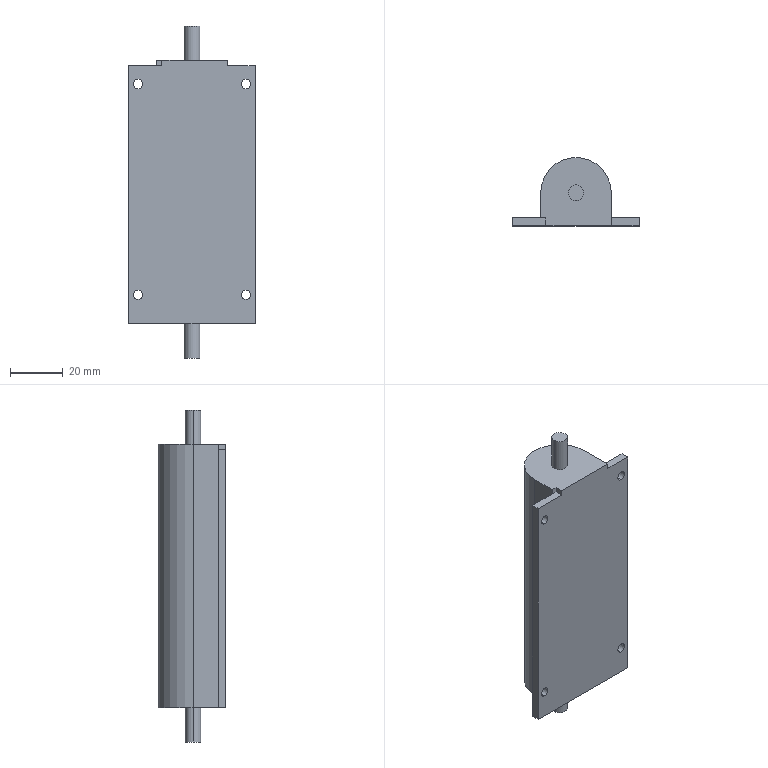Part | SolidWorks | features ICE 7, Extrusion 1 | 1 solid | 28 faces | box 48 x 25.9 x 126 mm | volume 68546 mm3 | plane 15 | cylinder 13 | commonest cylinder face diameters 3.5 x8 6 x4 26.8 x1
STEP:
#1=CARTESIAN_POINT('',(-20.5,3.,-38.25));
#2=VERTEX_POINT('',#1);
#3=CARTESIAN_POINT('',(-20.5,3.,-41.75));
#4=VERTEX_POINT('',#3);
#5=CARTESIAN_POINT('',(-20.5,3.,-40.));
#6=DIRECTION('',(0.,-1.,0.));
#7=DIRECTION('',(1.,0.,0.));
#8=AXIS2_PLACEMENT_3D('',#5,#6,#7);
#9=CIRCLE('',#8,1.75);
#10=EDGE_CURVE('',#2,#4,#9,.T.);
#11=ORIENTED_EDGE('',*,*,#10,.F.);
#12=CARTESIAN_POINT('',(-20.5,0.,-38.25));
#13=VERTEX_POINT('',#12);
#14=CARTESIAN_POINT('',(-20.5,10.,-38.25));
#15=DIRECTION('',(0.,-1.,0.));
#16=VECTOR('',#15,1000.);
#17=LINE('',#14,#16);
#18=EDGE_CURVE('',#2,#13,#17,.T.);
#19=ORIENTED_EDGE('',*,*,#18,.T.);
#20=CARTESIAN_POINT('',(-20.5,0.,-41.75));
#21=VERTEX_POINT('',#20);
#22=CARTESIAN_POINT('',(-20.5,0.,-40.));
#23=DIRECTION('',(0.,-1.,0.));
#24=DIRECTION('',(0.,0.,-1.));
#25=AXIS2_PLACEMENT_3D('',#22,#23,#24);
#26=CIRCLE('',#25,1.75);
#27=EDGE_CURVE('',#13,#21,#26,.T.);
#28=ORIENTED_EDGE('',*,*,#27,.T.);
#29=CARTESIAN_POINT('',(-20.5,10.,-41.75));
#30=DIRECTION('',(0.,-1.,0.));
#31=VECTOR('',#30,1000.);
#32=LINE('',#29,#31);
#33=EDGE_CURVE('',#4,#21,#32,.T.);
#34=ORIENTED_EDGE('',*,*,#33,.F.);
#35=EDGE_LOOP('',(#11,#19,#28,#34));
#36=FACE_OUTER_BOUND('',#35,.T.);
#37=CARTESIAN_POINT('',(-20.5,10.,-40.));
#38=DIRECTION('',(0.,-1.,0.));
#39=DIRECTION('',(0.,0.,-1.));
#40=AXIS2_PLACEMENT_3D('',#37,#38,#39);
#41=CYLINDRICAL_SURFACE('',#40,1.75);
#42=ADVANCED_FACE('',(#36),#41,.F.);
#43=CARTESIAN_POINT('',(20.5,3.,-38.25));
#44=VERTEX_POINT('',#43);
#45=CARTESIAN_POINT('',(20.5,3.,-41.75));
#46=VERTEX_POINT('',#45);
#47=CARTESIAN_POINT('',(20.5,3.,-40.));
#48=DIRECTION('',(0.,-1.,0.));
#49=DIRECTION('',(0.,0.,-1.));
#50=AXIS2_PLACEMENT_3D('',#47,#48,#49);
#51=CIRCLE('',#50,1.75);
#52=EDGE_CURVE('',#44,#46,#51,.T.);
#53=ORIENTED_EDGE('',*,*,#52,.F.);
#54=CARTESIAN_POINT('',(20.5,0.,-38.25));
#55=VERTEX_POINT('',#54);
#56=CARTESIAN_POINT('',(20.5,10.,-38.25));
#57=DIRECTION('',(0.,-1.,0.));
#58=VECTOR('',#57,1000.);
#59=LINE('',#56,#58);
#60=EDGE_CURVE('',#44,#55,#59,.T.);
#61=ORIENTED_EDGE('',*,*,#60,.T.);
#62=CARTESIAN_POINT('',(20.5,0.,-41.75));
#63=VERTEX_POINT('',#62);
#64=CARTESIAN_POINT('',(20.5,0.,-40.));
#65=DIRECTION('',(0.,-1.,0.));
#66=DIRECTION('',(0.,0.,-1.));
#67=AXIS2_PLACEMENT_3D('',#64,#65,#66);
#68=CIRCLE('',#67,1.75);
#69=EDGE_CURVE('',#55,#63,#68,.T.);
#70=ORIENTED_EDGE('',*,*,#69,.T.);
#71=CARTESIAN_POINT('',(20.5,10.,-41.75));
#72=DIRECTION('',(0.,-1.,0.));
#73=VECTOR('',#72,1000.);
#74=LINE('',#71,#73);
#75=EDGE_CURVE('',#46,#63,#74,.T.);
#76=ORIENTED_EDGE('',*,*,#75,.F.);
#77=EDGE_LOOP('',(#53,#61,#70,#76));
#78=FACE_OUTER_BOUND('',#77,.T.);
#79=CARTESIAN_POINT('',(20.5,10.,-40.));
#80=DIRECTION('',(0.,-1.,0.));
#81=DIRECTION('',(0.,0.,-1.));
#82=AXIS2_PLACEMENT_3D('',#79,#80,#81);
#83=CYLINDRICAL_SURFACE('',#82,1.75);
#84=ADVANCED_FACE('',(#78),#83,.F.);
#85=CARTESIAN_POINT('',(20.5,3.,41.75));
#86=VERTEX_POINT('',#85);
#87=CARTESIAN_POINT('',(20.5,3.,38.25));
#88=VERTEX_POINT('',#87);
#89=CARTESIAN_POINT('',(20.5,3.,40.));
#90=DIRECTION('',(0.,-1.,0.));
#91=DIRECTION('',(0.,0.,-1.));
#92=AXIS2_PLACEMENT_3D('',#89,#90,#91);
#93=CIRCLE('',#92,1.75);
#94=EDGE_CURVE('',#86,#88,#93,.T.);
#95=ORIENTED_EDGE('',*,*,#94,.F.);
#96=CARTESIAN_POINT('',(20.5,0.,41.75));
#97=VERTEX_POINT('',#96);
#98=CARTESIAN_POINT('',(20.5,10.,41.75));
#99=DIRECTION('',(0.,-1.,0.));
#100=VECTOR('',#99,1000.);
#101=LINE('',#98,#100);
#102=EDGE_CURVE('',#86,#97,#101,.T.);
#103=ORIENTED_EDGE('',*,*,#102,.T.);
#104=CARTESIAN_POINT('',(20.5,0.,38.25));
#105=VERTEX_POINT('',#104);
#106=CARTESIAN_POINT('',(20.5,0.,40.));
#107=DIRECTION('',(0.,-1.,0.));
#108=DIRECTION('',(0.,0.,-1.));
#109=AXIS2_PLACEMENT_3D('',#106,#107,#108);
#110=CIRCLE('',#109,1.75);
#111=EDGE_CURVE('',#97,#105,#110,.T.);
#112=ORIENTED_EDGE('',*,*,#111,.T.);
#113=CARTESIAN_POINT('',(20.5,10.,38.25));
#114=DIRECTION('',(0.,-1.,0.));
#115=VECTOR('',#114,1000.);
#116=LINE('',#113,#115);
#117=EDGE_CURVE('',#88,#105,#116,.T.);
#118=ORIENTED_EDGE('',*,*,#117,.F.);
#119=EDGE_LOOP('',(#95,#103,#112,#118));
#120=FACE_OUTER_BOUND('',#119,.T.);
#121=CARTESIAN_POINT('',(20.5,10.,40.));
#122=DIRECTION('',(0.,-1.,0.));
#123=DIRECTION('',(0.,0.,-1.));
#124=AXIS2_PLACEMENT_3D('',#121,#122,#123);
#125=CYLINDRICAL_SURFACE('',#124,1.75);
#126=ADVANCED_FACE('',(#120),#125,.F.);
#127=CARTESIAN_POINT('',(-20.5,3.,41.75));
#128=VERTEX_POINT('',#127);
#129=CARTESIAN_POINT('',(-20.5,3.,38.25));
#130=VERTEX_POINT('',#129);
#131=CARTESIAN_POINT('',(-20.5,3.,40.));
#132=DIRECTION('',(0.,-1.,0.));
#133=DIRECTION('',(1.,0.,0.));
#134=AXIS2_PLACEMENT_3D('',#131,#132,#133);
#135=CIRCLE('',#134,1.75);
#136=EDGE_CURVE('',#128,#130,#135,.T.);
#137=ORIENTED_EDGE('',*,*,#136,.F.);
#138=CARTESIAN_POINT('',(-20.5,0.,41.75));
#139=VERTEX_POINT('',#138);
#140=CARTESIAN_POINT('',(-20.5,10.,41.75));
#141=DIRECTION('',(0.,-1.,0.));
#142=VECTOR('',#141,1000.);
#143=LINE('',#140,#142);
#144=EDGE_CURVE('',#128,#139,#143,.T.);
#145=ORIENTED_EDGE('',*,*,#144,.T.);
#146=CARTESIAN_POINT('',(-20.5,0.,38.25));
#147=VERTEX_POINT('',#146);
#148=CARTESIAN_POINT('',(-20.5,0.,40.));
#149=DIRECTION('',(0.,-1.,0.));
#150=DIRECTION('',(0.,0.,-1.));
#151=AXIS2_PLACEMENT_3D('',#148,#149,#150);
#152=CIRCLE('',#151,1.75);
#153=EDGE_CURVE('',#139,#147,#152,.T.);
#154=ORIENTED_EDGE('',*,*,#153,.T.);
#155=CARTESIAN_POINT('',(-20.5,10.,38.25));
#156=DIRECTION('',(0.,-1.,0.));
#157=VECTOR('',#156,1000.);
#158=LINE('',#155,#157);
#159=EDGE_CURVE('',#130,#147,#158,.T.);
#160=ORIENTED_EDGE('',*,*,#159,.F.);
#161=EDGE_LOOP('',(#137,#145,#154,#160));
#162=FACE_OUTER_BOUND('',#161,.T.);
#163=CARTESIAN_POINT('',(-20.5,10.,40.));
#164=DIRECTION('',(0.,-1.,0.));
#165=DIRECTION('',(0.,0.,-1.));
#166=AXIS2_PLACEMENT_3D('',#163,#164,#165);
#167=CYLINDRICAL_SURFACE('',#166,1.75);
#168=ADVANCED_FACE('',(#162),#167,.F.);
#169=CARTESIAN_POINT('',(-3.,12.5,-64.));
#170=VERTEX_POINT('',#169);
#171=CARTESIAN_POINT('',(3.,12.5,-64.));
#172=VERTEX_POINT('',#171);
#173=CARTESIAN_POINT('',(0.,12.5,-64.));
#174=DIRECTION('',(0.,0.,-1.));
#175=DIRECTION('',(-1.,0.,0.));
#176=AXIS2_PLACEMENT_3D('',#173,#174,#175);
#177=CIRCLE('',#176,3.);
#178=EDGE_CURVE('',#170,#172,#177,.T.);
#179=ORIENTED_EDGE('',*,*,#178,.F.);
#180=CARTESIAN_POINT('',(-3.,12.5,-51.));
#181=VERTEX_POINT('',#180);
#182=CARTESIAN_POINT('',(-3.,12.5,-64.));
#183=DIRECTION('',(0.,0.,1.));
#184=VECTOR('',#183,1000.);
#185=LINE('',#182,#184);
#186=EDGE_CURVE('',#170,#181,#185,.T.);
#187=ORIENTED_EDGE('',*,*,#186,.T.);
#188=CARTESIAN_POINT('',(3.,12.5,-51.));
#189=VERTEX_POINT('',#188);
#190=CARTESIAN_POINT('',(0.,12.5,-51.));
#191=DIRECTION('',(0.,0.,-1.));
#192=DIRECTION('',(1.,0.,0.));
#193=AXIS2_PLACEMENT_3D('',#190,#191,#192);
#194=CIRCLE('',#193,3.);
#195=EDGE_CURVE('',#181,#189,#194,.T.);
#196=ORIENTED_EDGE('',*,*,#195,.T.);
#197=CARTESIAN_POINT('',(3.,12.5,-64.));
#198=DIRECTION('',(0.,0.,1.));
#199=VECTOR('',#198,1000.);
#200=LINE('',#197,#199);
#201=EDGE_CURVE('',#172,#189,#200,.T.);
#202=ORIENTED_EDGE('',*,*,#201,.F.);
#203=EDGE_LOOP('',(#179,#187,#196,#202));
#204=FACE_OUTER_BOUND('',#203,.T.);
#205=CARTESIAN_POINT('',(0.,12.5,-64.));
#206=DIRECTION('',(0.,0.,1.));
#207=DIRECTION('',(1.,0.,0.));
#208=AXIS2_PLACEMENT_3D('',#205,#206,#207);
#209=CYLINDRICAL_SURFACE('',#208,3.);
#210=ADVANCED_FACE('',(#204),#209,.T.);
#211=CARTESIAN_POINT('',(3.,12.5,62.));
#212=VERTEX_POINT('',#211);
#213=CARTESIAN_POINT('',(-3.,12.5,62.));
#214=VERTEX_POINT('',#213);
#215=CARTESIAN_POINT('',(0.,12.5,62.));
#216=DIRECTION('',(0.,0.,1.));
#217=DIRECTION('',(1.,0.,0.));
#218=AXIS2_PLACEMENT_3D('',#215,#216,#217);
#219=CIRCLE('',#218,3.);
#220=EDGE_CURVE('',#212,#214,#219,.T.);
#221=ORIENTED_EDGE('',*,*,#220,.F.);
#222=CARTESIAN_POINT('',(3.,12.5,49.));
#223=VERTEX_POINT('',#222);
#224=CARTESIAN_POINT('',(3.,12.5,62.));
#225=DIRECTION('',(0.,0.,-1.));
#226=VECTOR('',#225,1000.);
#227=LINE('',#224,#226);
#228=EDGE_CURVE('',#212,#223,#227,.T.);
#229=ORIENTED_EDGE('',*,*,#228,.T.);
#230=CARTESIAN_POINT('',(-3.,12.5,49.));
#231=VERTEX_POINT('',#230);
#232=CARTESIAN_POINT('',(0.,12.5,49.));
#233=DIRECTION('',(0.,0.,1.));
#234=DIRECTION('',(1.,0.,0.));
#235=AXIS2_PLACEMENT_3D('',#232,#233,#234);
#236=CIRCLE('',#235,3.);
#237=EDGE_CURVE('',#223,#231,#236,.T.);
#238=ORIENTED_EDGE('',*,*,#237,.T.);
#239=CARTESIAN_POINT('',(-3.,12.5,62.));
#240=DIRECTION('',(0.,0.,-1.));
#241=VECTOR('',#240,1000.);
#242=LINE('',#239,#241);
#243=EDGE_CURVE('',#214,#231,#242,.T.);
#244=ORIENTED_EDGE('',*,*,#243,.F.);
#245=EDGE_LOOP('',(#221,#229,#238,#244));
#246=FACE_OUTER_BOUND('',#245,.T.);
#247=CARTESIAN_POINT('',(0.,12.5,62.));
#248=DIRECTION('',(0.,0.,-1.));
#249=DIRECTION('',(-1.,0.,0.));
#250=AXIS2_PLACEMENT_3D('',#247,#248,#249);
#251=CYLINDRICAL_SURFACE('',#250,3.);
#252=ADVANCED_FACE('',(#246),#251,.T.);
#253=CARTESIAN_POINT('',(-24.,3.,-51.));
#254=VERTEX_POINT('',#253);
#255=CARTESIAN_POINT('',(-24.,0.,-51.));
#256=VERTEX_POINT('',#255);
#257=CARTESIAN_POINT('',(-24.,0.,-51.));
#258=DIRECTION('',(0.,-1.,0.));
#259=VECTOR('',#258,1000.);
#260=LINE('',#257,#259);
#261=EDGE_CURVE('',#254,#256,#260,.T.);
#262=ORIENTED_EDGE('',*,*,#261,.F.);
#263=CARTESIAN_POINT('',(-13.4,3.,-51.));
#264=VERTEX_POINT('',#263);
#265=CARTESIAN_POINT('',(-13.4,3.,-51.));
#266=DIRECTION('',(-1.,0.,0.));
#267=VECTOR('',#266,1000.);
#268=LINE('',#265,#267);
#269=EDGE_CURVE('',#264,#254,#268,.T.);
#270=ORIENTED_EDGE('',*,*,#269,.F.);
#271=CARTESIAN_POINT('',(-13.4,12.5,-51.));
#272=VERTEX_POINT('',#271);
#273=CARTESIAN_POINT('',(-13.4,12.5,-51.));
#274=DIRECTION('',(0.,-1.,0.));
#275=VECTOR('',#274,1000.);
#276=LINE('',#273,#275);
#277=EDGE_CURVE('',#272,#264,#276,.T.);
#278=ORIENTED_EDGE('',*,*,#277,.F.);
#279=CARTESIAN_POINT('',(13.4,12.5,-51.));
#280=VERTEX_POINT('',#279);
#281=CARTESIAN_POINT('',(0.,12.5,-51.));
#282=DIRECTION('',(0.,0.,1.));
#283=DIRECTION('',(1.,0.,0.));
#284=AXIS2_PLACEMENT_3D('',#281,#282,#283);
#285=CIRCLE('',#284,13.4);
#286=EDGE_CURVE('',#280,#272,#285,.T.);
#287=ORIENTED_EDGE('',*,*,#286,.F.);
#288=CARTESIAN_POINT('',(13.4,3.,-51.));
#289=VERTEX_POINT('',#288);
#290=CARTESIAN_POINT('',(13.4,0.,-51.));
#291=DIRECTION('',(0.,1.,0.));
#292=VECTOR('',#291,1000.);
#293=LINE('',#290,#292);
#294=EDGE_CURVE('',#289,#280,#293,.T.);
#295=ORIENTED_EDGE('',*,*,#294,.F.);
#296=CARTESIAN_POINT('',(24.,3.,-51.));
#297=VERTEX_POINT('',#296);
#298=CARTESIAN_POINT('',(24.,3.,-51.));
#299=DIRECTION('',(-1.,0.,0.));
#300=VECTOR('',#299,1000.);
#301=LINE('',#298,#300);
#302=EDGE_CURVE('',#297,#289,#301,.T.);
#303=ORIENTED_EDGE('',*,*,#302,.F.);
#304=CARTESIAN_POINT('',(24.,0.,-51.));
#305=VERTEX_POINT('',#304);
#306=CARTESIAN_POINT('',(24.,3.,-51.));
#307=DIRECTION('',(0.,1.,0.));
#308=VECTOR('',#307,1000.);
#309=LINE('',#306,#308);
#310=EDGE_CURVE('',#305,#297,#309,.T.);
#311=ORIENTED_EDGE('',*,*,#310,.F.);
#312=CARTESIAN_POINT('',(-13.4,0.,-51.));
#313=DIRECTION('',(1.,0.,0.));
#314=VECTOR('',#313,1000.);
#315=LINE('',#312,#314);
#316=EDGE_CURVE('',#256,#305,#315,.T.);
#317=ORIENTED_EDGE('',*,*,#316,.F.);
#318=EDGE_LOOP('',(#262,#270,#278,#287,#295,#303,#311,#317));
#319=FACE_OUTER_BOUND('',#318,.T.);
#320=CARTESIAN_POINT('',(0.,12.5,-51.));
#321=DIRECTION('',(0.,0.,-1.));
#322=DIRECTION('',(1.,0.,0.));
#323=AXIS2_PLACEMENT_3D('',#320,#321,#322);
#324=CIRCLE('',#323,3.);
#325=EDGE_CURVE('',#189,#181,#324,.T.);
#326=ORIENTED_EDGE('',*,*,#325,.F.);
#327=ORIENTED_EDGE('',*,*,#195,.F.);
#328=EDGE_LOOP('',(#326,#327));
#329=FACE_BOUND('',#328,.T.);
#330=CARTESIAN_POINT('',(0.,12.5,-51.));
#331=DIRECTION('',(0.,0.,1.));
#332=DIRECTION('',(1.,0.,0.));
#333=AXIS2_PLACEMENT_3D('',#330,#331,#332);
#334=PLANE('',#333);
#335=ADVANCED_FACE('',(#319,#329),#334,.F.);
#336=CARTESIAN_POINT('',(-11.4,3.,49.));
#337=VERTEX_POINT('',#336);
#338=CARTESIAN_POINT('',(-13.4,3.,49.));
#339=VERTEX_POINT('',#338);
#340=CARTESIAN_POINT('',(-11.4,3.,49.));
#341=DIRECTION('',(-1.,0.,0.));
#342=VECTOR('',#341,1000.);
#343=LINE('',#340,#342);
#344=EDGE_CURVE('',#337,#339,#343,.T.);
#345=ORIENTED_EDGE('',*,*,#344,.F.);
#346=CARTESIAN_POINT('',(-11.4,0.,49.));
#347=VERTEX_POINT('',#346);
#348=CARTESIAN_POINT('',(-11.4,12.5,49.));
#349=DIRECTION('',(0.,1.,0.));
#350=VECTOR('',#349,1000.);
#351=LINE('',#348,#350);
#352=EDGE_CURVE('',#347,#337,#351,.T.);
#353=ORIENTED_EDGE('',*,*,#352,.F.);
#354=CARTESIAN_POINT('',(13.4,0.,49.));
#355=VERTEX_POINT('',#354);
#356=CARTESIAN_POINT('',(-13.4,0.,49.));
#357=DIRECTION('',(1.,0.,0.));
#358=VECTOR('',#357,1000.);
#359=LINE('',#356,#358);
#360=EDGE_CURVE('',#347,#355,#359,.T.);
#361=ORIENTED_EDGE('',*,*,#360,.T.);
#362=CARTESIAN_POINT('',(13.4,12.5,49.));
#363=VERTEX_POINT('',#362);
#364=CARTESIAN_POINT('',(13.4,0.,49.));
#365=DIRECTION('',(0.,1.,0.));
#366=VECTOR('',#365,1000.);
#367=LINE('',#364,#366);
#368=EDGE_CURVE('',#355,#363,#367,.T.);
#369=ORIENTED_EDGE('',*,*,#368,.T.);
#370=CARTESIAN_POINT('',(-13.4,12.5,49.));
#371=VERTEX_POINT('',#370);
#372=CARTESIAN_POINT('',(0.,12.5,49.));
#373=DIRECTION('',(0.,0.,1.));
#374=DIRECTION('',(1.,0.,0.));
#375=AXIS2_PLACEMENT_3D('',#372,#373,#374);
#376=CIRCLE('',#375,13.4);
#377=EDGE_CURVE('',#363,#371,#376,.T.);
#378=ORIENTED_EDGE('',*,*,#377,.T.);
#379=CARTESIAN_POINT('',(-13.4,12.5,49.));
#380=DIRECTION('',(0.,-1.,0.));
#381=VECTOR('',#380,1000.);
#382=LINE('',#379,#381);
#383=EDGE_CURVE('',#371,#339,#382,.T.);
#384=ORIENTED_EDGE('',*,*,#383,.T.);
#385=EDGE_LOOP('',(#345,#353,#361,#369,#378,#384));
#386=FACE_OUTER_BOUND('',#385,.T.);
#387=CARTESIAN_POINT('',(0.,12.5,49.));
#388=DIRECTION('',(0.,0.,1.));
#389=DIRECTION('',(1.,0.,0.));
#390=AXIS2_PLACEMENT_3D('',#387,#388,#389);
#391=CIRCLE('',#390,3.);
#392=EDGE_CURVE('',#231,#223,#391,.T.);
#393=ORIENTED_EDGE('',*,*,#392,.F.);
#394=ORIENTED_EDGE('',*,*,#237,.F.);
#395=EDGE_LOOP('',(#393,#394));
#396=FACE_BOUND('',#395,.T.);
#397=CARTESIAN_POINT('',(0.,12.5,49.));
#398=DIRECTION('',(0.,0.,1.));
#399=DIRECTION('',(1.,0.,0.));
#400=AXIS2_PLACEMENT_3D('',#397,#398,#399);
#401=PLANE('',#400);
#402=ADVANCED_FACE('',(#386,#396),#401,.T.);
#403=CARTESIAN_POINT('',(-13.4,3.,47.));
#404=VERTEX_POINT('',#403);
#405=CARTESIAN_POINT('',(-13.4,3.,-51.));
#406=DIRECTION('',(0.,0.,1.));
#407=VECTOR('',#406,1000.);
#408=LINE('',#405,#407);
#409=EDGE_CURVE('',#404,#339,#408,.T.);
#410=ORIENTED_EDGE('',*,*,#409,.T.);
#411=ORIENTED_EDGE('',*,*,#383,.F.);
#412=CARTESIAN_POINT('',(-13.4,12.5,-51.));
#413=DIRECTION('',(0.,0.,1.));
#414=VECTOR('',#413,1000.);
#415=LINE('',#412,#414);
#416=EDGE_CURVE('',#272,#371,#415,.T.);
#417=ORIENTED_EDGE('',*,*,#416,.F.);
#418=ORIENTED_EDGE('',*,*,#277,.T.);
#419=CARTESIAN_POINT('',(-13.4,3.,49.));
#420=DIRECTION('',(0.,0.,-1.));
#421=VECTOR('',#420,1000.);
#422=LINE('',#419,#421);
#423=EDGE_CURVE('',#404,#264,#422,.T.);
#424=ORIENTED_EDGE('',*,*,#423,.F.);
#425=EDGE_LOOP('',(#410,#411,#417,#418,#424));
#426=FACE_OUTER_BOUND('',#425,.T.);
#427=CARTESIAN_POINT('',(-13.4,12.5,-51.));
#428=DIRECTION('',(-1.,0.,0.));
#429=DIRECTION('',(0.,0.,1.));
#430=AXIS2_PLACEMENT_3D('',#427,#428,#429);
#431=PLANE('',#430);
#432=ADVANCED_FACE('',(#426),#431,.T.);
#433=CARTESIAN_POINT('',(-11.4,3.,47.));
#434=VERTEX_POINT('',#433);
#435=CARTESIAN_POINT('',(-11.4,3.,47.));
#436=DIRECTION('',(-1.,0.,0.));
#437=VECTOR('',#436,1000.);
#438=LINE('',#435,#437);
#439=EDGE_CURVE('',#434,#404,#438,.T.);
#440=ORIENTED_EDGE('',*,*,#439,.F.);
#441=CARTESIAN_POINT('',(-11.4,3.,-51.));
#442=DIRECTION('',(0.,0.,1.));
#443=VECTOR('',#442,1000.);
#444=LINE('',#441,#443);
#445=EDGE_CURVE('',#434,#337,#444,.T.);
#446=ORIENTED_EDGE('',*,*,#445,.T.);
#447=ORIENTED_EDGE('',*,*,#344,.T.);
#448=ORIENTED_EDGE('',*,*,#409,.F.);
#449=EDGE_LOOP('',(#440,#446,#447,#448));
#450=FACE_OUTER_BOUND('',#449,.T.);
#451=CARTESIAN_POINT('',(-11.4,3.,-51.));
#452=DIRECTION('',(0.,1.,0.));
#453=DIRECTION('',(-1.,0.,0.));
#454=AXIS2_PLACEMENT_3D('',#451,#452,#453);
#455=PLANE('',#454);
#456=ADVANCED_FACE('',(#450),#455,.F.);
#457=CARTESIAN_POINT('',(-11.4,0.,47.));
#458=VERTEX_POINT('',#457);
#459=CARTESIAN_POINT('',(-11.4,4.9,47.));
#460=DIRECTION('',(0.,1.,0.));
#461=VECTOR('',#460,1000.);
#462=LINE('',#459,#461);
#463=EDGE_CURVE('',#458,#434,#462,.T.);
#464=ORIENTED_EDGE('',*,*,#463,.F.);
#465=CARTESIAN_POINT('',(-11.4,0.,-51.));
#466=DIRECTION('',(0.,0.,1.));
#467=VECTOR('',#466,1000.);
#468=LINE('',#465,#467);
#469=EDGE_CURVE('',#458,#347,#468,.T.);
#470=ORIENTED_EDGE('',*,*,#469,.T.);
#471=ORIENTED_EDGE('',*,*,#352,.T.);
#472=ORIENTED_EDGE('',*,*,#445,.F.);
#473=EDGE_LOOP('',(#464,#470,#471,#472));
#474=FACE_OUTER_BOUND('',#473,.T.);
#475=CARTESIAN_POINT('',(-11.4,-3.4,-51.));
#476=DIRECTION('',(1.,0.,0.));
#477=DIRECTION('',(0.,0.,-1.));
#478=AXIS2_PLACEMENT_3D('',#475,#476,#477);
#479=PLANE('',#478);
#480=ADVANCED_FACE('',(#474),#479,.F.);
#481=CARTESIAN_POINT('',(13.4,3.,47.));
#482=VERTEX_POINT('',#481);
#483=CARTESIAN_POINT('',(13.4,0.,47.));
#484=VERTEX_POINT('',#483);
#485=CARTESIAN_POINT('',(13.4,0.,47.));
#486=DIRECTION('',(0.,-1.,0.));
#487=VECTOR('',#486,1000.);
#488=LINE('',#485,#487);
#489=EDGE_CURVE('',#482,#484,#488,.T.);
#490=ORIENTED_EDGE('',*,*,#489,.F.);
#491=CARTESIAN_POINT('',(13.4,3.,47.));
#492=DIRECTION('',(0.,0.,1.));
#493=VECTOR('',#492,1000.);
#494=LINE('',#491,#493);
#495=EDGE_CURVE('',#289,#482,#494,.T.);
#496=ORIENTED_EDGE('',*,*,#495,.F.);
#497=ORIENTED_EDGE('',*,*,#294,.T.);
#498=CARTESIAN_POINT('',(13.4,12.5,-51.));
#499=DIRECTION('',(0.,0.,1.));
#500=VECTOR('',#499,1000.);
#501=LINE('',#498,#500);
#502=EDGE_CURVE('',#280,#363,#501,.T.);
#503=ORIENTED_EDGE('',*,*,#502,.T.);
#504=ORIENTED_EDGE('',*,*,#368,.F.);
#505=CARTESIAN_POINT('',(13.4,0.,-51.));
#506=DIRECTION('',(0.,0.,1.));
#507=VECTOR('',#506,1000.);
#508=LINE('',#505,#507);
#509=EDGE_CURVE('',#484,#355,#508,.T.);
#510=ORIENTED_EDGE('',*,*,#509,.F.);
#511=EDGE_LOOP('',(#490,#496,#497,#503,#504,#510));
#512=FACE_OUTER_BOUND('',#511,.T.);
#513=CARTESIAN_POINT('',(13.4,0.,-51.));
#514=DIRECTION('',(1.,0.,0.));
#515=DIRECTION('',(0.,0.,-1.));
#516=AXIS2_PLACEMENT_3D('',#513,#514,#515);
#517=PLANE('',#516);
#518=ADVANCED_FACE('',(#512),#517,.T.);
#519=ORIENTED_EDGE('',*,*,#377,.F.);
#520=ORIENTED_EDGE('',*,*,#502,.F.);
#521=ORIENTED_EDGE('',*,*,#286,.T.);
#522=ORIENTED_EDGE('',*,*,#416,.T.);
#523=EDGE_LOOP('',(#519,#520,#521,#522));
#524=FACE_OUTER_BOUND('',#523,.T.);
#525=CARTESIAN_POINT('',(0.,12.5,-51.));
#526=DIRECTION('',(0.,0.,1.));
#527=DIRECTION('',(1.,0.,0.));
#528=AXIS2_PLACEMENT_3D('',#525,#526,#527);
#529=CYLINDRICAL_SURFACE('',#528,13.4);
#530=ADVANCED_FACE('',(#524),#529,.T.);
#531=CARTESIAN_POINT('',(-20.5,0.,-40.));
#532=DIRECTION('',(0.,-1.,0.));
#533=DIRECTION('',(0.,0.,-1.));
#534=AXIS2_PLACEMENT_3D('',#531,#532,#533);
#535=CIRCLE('',#534,1.75);
#536=EDGE_CURVE('',#21,#13,#535,.T.);
#537=ORIENTED_EDGE('',*,*,#536,.F.);
#538=ORIENTED_EDGE('',*,*,#27,.F.);
#539=EDGE_LOOP('',(#537,#538));
#540=FACE_BOUND('',#539,.T.);
#541=CARTESIAN_POINT('',(20.5,0.,-40.));
#542=DIRECTION('',(0.,-1.,0.));
#543=DIRECTION('',(0.,0.,-1.));
#544=AXIS2_PLACEMENT_3D('',#541,#542,#543);
#545=CIRCLE('',#544,1.75);
#546=EDGE_CURVE('',#63,#55,#545,.T.);
#547=ORIENTED_EDGE('',*,*,#546,.F.);
#548=ORIENTED_EDGE('',*,*,#69,.F.);
#549=EDGE_LOOP('',(#547,#548));
#550=FACE_BOUND('',#549,.T.);
#551=CARTESIAN_POINT('',(20.5,0.,40.));
#552=DIRECTION('',(0.,-1.,0.));
#553=DIRECTION('',(0.,0.,-1.));
#554=AXIS2_PLACEMENT_3D('',#551,#552,#553);
#555=CIRCLE('',#554,1.75);
#556=EDGE_CURVE('',#105,#97,#555,.T.);
#557=ORIENTED_EDGE('',*,*,#556,.F.);
#558=ORIENTED_EDGE('',*,*,#111,.F.);
#559=EDGE_LOOP('',(#557,#558));
#560=FACE_BOUND('',#559,.T.);
#561=CARTESIAN_POINT('',(-20.5,0.,40.));
#562=DIRECTION('',(0.,-1.,0.));
#563=DIRECTION('',(0.,0.,-1.));
#564=AXIS2_PLACEMENT_3D('',#561,#562,#563);
#565=CIRCLE('',#564,1.75);
#566=EDGE_CURVE('',#147,#139,#565,.T.);
#567=ORIENTED_EDGE('',*,*,#566,.F.);
#568=ORIENTED_EDGE('',*,*,#153,.F.);
#569=EDGE_LOOP('',(#567,#568));
#570=FACE_BOUND('',#569,.T.);
#571=ORIENTED_EDGE('',*,*,#469,.F.);
#572=CARTESIAN_POINT('',(-24.,0.,47.));
#573=VERTEX_POINT('',#572);
#574=CARTESIAN_POINT('',(-24.,0.,47.));
#575=DIRECTION('',(1.,0.,0.));
#576=VECTOR('',#575,1000.);
#577=LINE('',#574,#576);
#578=EDGE_CURVE('',#573,#458,#577,.T.);
#579=ORIENTED_EDGE('',*,*,#578,.F.);
#580=CARTESIAN_POINT('',(-24.,0.,47.));
#581=DIRECTION('',(0.,0.,1.));
#582=VECTOR('',#581,1000.);
#583=LINE('',#580,#582);
#584=EDGE_CURVE('',#256,#573,#583,.T.);
#585=ORIENTED_EDGE('',*,*,#584,.F.);
#586=ORIENTED_EDGE('',*,*,#316,.T.);
#587=CARTESIAN_POINT('',(24.,0.,47.));
#588=VERTEX_POINT('',#587);
#589=CARTESIAN_POINT('',(24.,0.,-51.));
#590=DIRECTION('',(0.,0.,-1.));
#591=VECTOR('',#590,1000.);
#592=LINE('',#589,#591);
#593=EDGE_CURVE('',#588,#305,#592,.T.);
#594=ORIENTED_EDGE('',*,*,#593,.F.);
#595=CARTESIAN_POINT('',(24.,0.,47.));
#596=DIRECTION('',(-1.,0.,0.));
#597=VECTOR('',#596,1000.);
#598=LINE('',#595,#597);
#599=EDGE_CURVE('',#588,#484,#598,.T.);
#600=ORIENTED_EDGE('',*,*,#599,.T.);
#601=ORIENTED_EDGE('',*,*,#509,.T.);
#602=ORIENTED_EDGE('',*,*,#360,.F.);
#603=EDGE_LOOP('',(#571,#579,#585,#586,#594,#600,#601,#602));
#604=FACE_OUTER_BOUND('',#603,.T.);
#605=CARTESIAN_POINT('',(-13.4,0.,-51.));
#606=DIRECTION('',(0.,-1.,0.));
#607=DIRECTION('',(0.,0.,-1.));
#608=AXIS2_PLACEMENT_3D('',#605,#606,#607);
#609=PLANE('',#608);
#610=ADVANCED_FACE('',(#540,#550,#560,#570,#604),#609,.T.);
#611=CARTESIAN_POINT('',(20.5,3.,-40.));
#612=DIRECTION('',(0.,-1.,0.));
#613=DIRECTION('',(0.,0.,-1.));
#614=AXIS2_PLACEMENT_3D('',#611,#612,#613);
#615=CIRCLE('',#614,1.75);
#616=EDGE_CURVE('',#46,#44,#615,.T.);
#617=ORIENTED_EDGE('',*,*,#616,.T.);
#618=ORIENTED_EDGE('',*,*,#52,.T.);
#619=EDGE_LOOP('',(#617,#618));
#620=FACE_BOUND('',#619,.T.);
#621=CARTESIAN_POINT('',(20.5,3.,40.));
#622=DIRECTION('',(0.,-1.,0.));
#623=DIRECTION('',(0.,0.,-1.));
#624=AXIS2_PLACEMENT_3D('',#621,#622,#623);
#625=CIRCLE('',#624,1.75);
#626=EDGE_CURVE('',#88,#86,#625,.T.);
#627=ORIENTED_EDGE('',*,*,#626,.T.);
#628=ORIENTED_EDGE('',*,*,#94,.T.);
#629=EDGE_LOOP('',(#627,#628));
#630=FACE_BOUND('',#629,.T.);
#631=ORIENTED_EDGE('',*,*,#495,.T.);
#632=CARTESIAN_POINT('',(24.,3.,47.));
#633=VERTEX_POINT('',#632);
#634=CARTESIAN_POINT('',(24.,3.,47.));
#635=DIRECTION('',(-1.,0.,0.));
#636=VECTOR('',#635,1000.);
#637=LINE('',#634,#636);
#638=EDGE_CURVE('',#633,#482,#637,.T.);
#639=ORIENTED_EDGE('',*,*,#638,.F.);
#640=CARTESIAN_POINT('',(24.,3.,47.));
#641=DIRECTION('',(0.,0.,1.));
#642=VECTOR('',#641,1000.);
#643=LINE('',#640,#642);
#644=EDGE_CURVE('',#297,#633,#643,.T.);
#645=ORIENTED_EDGE('',*,*,#644,.F.);
#646=ORIENTED_EDGE('',*,*,#302,.T.);
#647=EDGE_LOOP('',(#631,#639,#645,#646));
#648=FACE_OUTER_BOUND('',#647,.T.);
#649=CARTESIAN_POINT('',(24.,3.,47.));
#650=DIRECTION('',(0.,-1.,0.));
#651=DIRECTION('',(0.,0.,-1.));
#652=AXIS2_PLACEMENT_3D('',#649,#650,#651);
#653=PLANE('',#652);
#654=ADVANCED_FACE('',(#620,#630,#648),#653,.F.);
#655=ORIENTED_EDGE('',*,*,#489,.T.);
#656=ORIENTED_EDGE('',*,*,#599,.F.);
#657=CARTESIAN_POINT('',(24.,0.,47.));
#658=DIRECTION('',(0.,-1.,0.));
#659=VECTOR('',#658,1000.);
#660=LINE('',#657,#659);
#661=EDGE_CURVE('',#633,#588,#660,.T.);
#662=ORIENTED_EDGE('',*,*,#661,.F.);
#663=ORIENTED_EDGE('',*,*,#638,.T.);
#664=EDGE_LOOP('',(#655,#656,#662,#663));
#665=FACE_OUTER_BOUND('',#664,.T.);
#666=CARTESIAN_POINT('',(24.,0.,47.));
#667=DIRECTION('',(0.,0.,-1.));
#668=DIRECTION('',(-1.,0.,0.));
#669=AXIS2_PLACEMENT_3D('',#666,#667,#668);
#670=PLANE('',#669);
#671=ADVANCED_FACE('',(#665),#670,.F.);
#672=ORIENTED_EDGE('',*,*,#310,.T.);
#673=ORIENTED_EDGE('',*,*,#644,.T.);
#674=ORIENTED_EDGE('',*,*,#661,.T.);
#675=ORIENTED_EDGE('',*,*,#593,.T.);
#676=EDGE_LOOP('',(#672,#673,#674,#675));
#677=FACE_OUTER_BOUND('',#676,.T.);
#678=CARTESIAN_POINT('',(24.,0.,0.));
#679=DIRECTION('',(-1.,0.,0.));
#680=DIRECTION('',(0.,0.,1.));
#681=AXIS2_PLACEMENT_3D('',#678,#679,#680);
#682=PLANE('',#681);
#683=ADVANCED_FACE('',(#677),#682,.F.);
#684=ORIENTED_EDGE('',*,*,#439,.T.);
#685=CARTESIAN_POINT('',(-24.,3.,47.));
#686=VERTEX_POINT('',#685);
#687=CARTESIAN_POINT('',(-24.,3.,47.));
#688=DIRECTION('',(-1.,0.,0.));
#689=VECTOR('',#688,1000.);
#690=LINE('',#687,#689);
#691=EDGE_CURVE('',#404,#686,#690,.T.);
#692=ORIENTED_EDGE('',*,*,#691,.T.);
#693=CARTESIAN_POINT('',(-24.,4.9,47.));
#694=DIRECTION('',(0.,1.,0.));
#695=VECTOR('',#694,1000.);
#696=LINE('',#693,#695);
#697=EDGE_CURVE('',#573,#686,#696,.T.);
#698=ORIENTED_EDGE('',*,*,#697,.F.);
#699=ORIENTED_EDGE('',*,*,#578,.T.);
#700=ORIENTED_EDGE('',*,*,#463,.T.);
#701=EDGE_LOOP('',(#684,#692,#698,#699,#700));
#702=FACE_OUTER_BOUND('',#701,.T.);
#703=CARTESIAN_POINT('',(-24.,4.9,47.));
#704=DIRECTION('',(0.,0.,-1.));
#705=DIRECTION('',(-1.,0.,0.));
#706=AXIS2_PLACEMENT_3D('',#703,#704,#705);
#707=PLANE('',#706);
#708=ADVANCED_FACE('',(#702),#707,.F.);
#709=ORIENTED_EDGE('',*,*,#697,.T.);
#710=CARTESIAN_POINT('',(-24.,3.,0.));
#711=DIRECTION('',(0.,0.,-1.));
#712=VECTOR('',#711,1000.);
#713=LINE('',#710,#712);
#714=EDGE_CURVE('',#686,#254,#713,.T.);
#715=ORIENTED_EDGE('',*,*,#714,.T.);
#716=ORIENTED_EDGE('',*,*,#261,.T.);
#717=ORIENTED_EDGE('',*,*,#584,.T.);
#718=EDGE_LOOP('',(#709,#715,#716,#717));
#719=FACE_OUTER_BOUND('',#718,.T.);
#720=CARTESIAN_POINT('',(-24.,0.,0.));
#721=DIRECTION('',(1.,0.,0.));
#722=DIRECTION('',(0.,0.,-1.));
#723=AXIS2_PLACEMENT_3D('',#720,#721,#722);
#724=PLANE('',#723);
#725=ADVANCED_FACE('',(#719),#724,.F.);
#726=CARTESIAN_POINT('',(-20.5,3.,-40.));
#727=DIRECTION('',(0.,-1.,0.));
#728=DIRECTION('',(1.,0.,0.));
#729=AXIS2_PLACEMENT_3D('',#726,#727,#728);
#730=CIRCLE('',#729,1.75);
#731=EDGE_CURVE('',#4,#2,#730,.T.);
#732=ORIENTED_EDGE('',*,*,#731,.T.);
#733=ORIENTED_EDGE('',*,*,#10,.T.);
#734=EDGE_LOOP('',(#732,#733));
#735=FACE_BOUND('',#734,.T.);
#736=CARTESIAN_POINT('',(-20.5,3.,40.));
#737=DIRECTION('',(0.,-1.,0.));
#738=DIRECTION('',(1.,0.,0.));
#739=AXIS2_PLACEMENT_3D('',#736,#737,#738);
#740=CIRCLE('',#739,1.75);
#741=EDGE_CURVE('',#130,#128,#740,.T.);
#742=ORIENTED_EDGE('',*,*,#741,.T.);
#743=ORIENTED_EDGE('',*,*,#136,.T.);
#744=EDGE_LOOP('',(#742,#743));
#745=FACE_BOUND('',#744,.T.);
#746=ORIENTED_EDGE('',*,*,#423,.T.);
#747=ORIENTED_EDGE('',*,*,#269,.T.);
#748=ORIENTED_EDGE('',*,*,#714,.F.);
#749=ORIENTED_EDGE('',*,*,#691,.F.);
#750=EDGE_LOOP('',(#746,#747,#748,#749));
#751=FACE_OUTER_BOUND('',#750,.T.);
#752=CARTESIAN_POINT('',(-13.4,3.,49.));
#753=DIRECTION('',(0.,-1.,0.));
#754=DIRECTION('',(1.,0.,0.));
#755=AXIS2_PLACEMENT_3D('',#752,#753,#754);
#756=PLANE('',#755);
#757=ADVANCED_FACE('',(#735,#745,#751),#756,.F.);
#758=ORIENTED_EDGE('',*,*,#228,.F.);
#759=CARTESIAN_POINT('',(0.,12.5,62.));
#760=DIRECTION('',(0.,0.,1.));
#761=DIRECTION('',(1.,0.,0.));
#762=AXIS2_PLACEMENT_3D('',#759,#760,#761);
#763=CIRCLE('',#762,3.);
#764=EDGE_CURVE('',#214,#212,#763,.T.);
#765=ORIENTED_EDGE('',*,*,#764,.F.);
#766=ORIENTED_EDGE('',*,*,#243,.T.);
#767=ORIENTED_EDGE('',*,*,#392,.T.);
#768=EDGE_LOOP('',(#758,#765,#766,#767));
#769=FACE_OUTER_BOUND('',#768,.T.);
#770=CARTESIAN_POINT('',(0.,12.5,62.));
#771=DIRECTION('',(0.,0.,-1.));
#772=DIRECTION('',(-1.,0.,0.));
#773=AXIS2_PLACEMENT_3D('',#770,#771,#772);
#774=CYLINDRICAL_SURFACE('',#773,3.);
#775=ADVANCED_FACE('',(#769),#774,.T.);
#776=ORIENTED_EDGE('',*,*,#764,.T.);
#777=ORIENTED_EDGE('',*,*,#220,.T.);
#778=EDGE_LOOP('',(#776,#777));
#779=FACE_OUTER_BOUND('',#778,.T.);
#780=CARTESIAN_POINT('',(0.,12.5,62.));
#781=DIRECTION('',(0.,0.,1.));
#782=DIRECTION('',(1.,0.,0.));
#783=AXIS2_PLACEMENT_3D('',#780,#781,#782);
#784=PLANE('',#783);
#785=ADVANCED_FACE('',(#779),#784,.T.);
#786=ORIENTED_EDGE('',*,*,#186,.F.);
#787=CARTESIAN_POINT('',(0.,12.5,-64.));
#788=DIRECTION('',(0.,0.,-1.));
#789=DIRECTION('',(-1.,0.,0.));
#790=AXIS2_PLACEMENT_3D('',#787,#788,#789);
#791=CIRCLE('',#790,3.);
#792=EDGE_CURVE('',#172,#170,#791,.T.);
#793=ORIENTED_EDGE('',*,*,#792,.F.);
#794=ORIENTED_EDGE('',*,*,#201,.T.);
#795=ORIENTED_EDGE('',*,*,#325,.T.);
#796=EDGE_LOOP('',(#786,#793,#794,#795));
#797=FACE_OUTER_BOUND('',#796,.T.);
#798=CARTESIAN_POINT('',(0.,12.5,-64.));
#799=DIRECTION('',(0.,0.,1.));
#800=DIRECTION('',(1.,0.,0.));
#801=AXIS2_PLACEMENT_3D('',#798,#799,#800);
#802=CYLINDRICAL_SURFACE('',#801,3.);
#803=ADVANCED_FACE('',(#797),#802,.T.);
#804=ORIENTED_EDGE('',*,*,#792,.T.);
#805=ORIENTED_EDGE('',*,*,#178,.T.);
#806=EDGE_LOOP('',(#804,#805));
#807=FACE_OUTER_BOUND('',#806,.T.);
#808=CARTESIAN_POINT('',(0.,12.5,-64.));
#809=DIRECTION('',(0.,0.,-1.));
#810=DIRECTION('',(-1.,0.,0.));
#811=AXIS2_PLACEMENT_3D('',#808,#809,#810);
#812=PLANE('',#811);
#813=ADVANCED_FACE('',(#807),#812,.T.);
#814=ORIENTED_EDGE('',*,*,#144,.F.);
#815=ORIENTED_EDGE('',*,*,#741,.F.);
#816=ORIENTED_EDGE('',*,*,#159,.T.);
#817=ORIENTED_EDGE('',*,*,#566,.T.);
#818=EDGE_LOOP('',(#814,#815,#816,#817));
#819=FACE_OUTER_BOUND('',#818,.T.);
#820=CARTESIAN_POINT('',(-20.5,10.,40.));
#821=DIRECTION('',(0.,-1.,0.));
#822=DIRECTION('',(0.,0.,-1.));
#823=AXIS2_PLACEMENT_3D('',#820,#821,#822);
#824=CYLINDRICAL_SURFACE('',#823,1.75);
#825=ADVANCED_FACE('',(#819),#824,.F.);
#826=ORIENTED_EDGE('',*,*,#102,.F.);
#827=ORIENTED_EDGE('',*,*,#626,.F.);
#828=ORIENTED_EDGE('',*,*,#117,.T.);
#829=ORIENTED_EDGE('',*,*,#556,.T.);
#830=EDGE_LOOP('',(#826,#827,#828,#829));
#831=FACE_OUTER_BOUND('',#830,.T.);
#832=CARTESIAN_POINT('',(20.5,10.,40.));
#833=DIRECTION('',(0.,-1.,0.));
#834=DIRECTION('',(0.,0.,-1.));
#835=AXIS2_PLACEMENT_3D('',#832,#833,#834);
#836=CYLINDRICAL_SURFACE('',#835,1.75);
#837=ADVANCED_FACE('',(#831),#836,.F.);
#838=ORIENTED_EDGE('',*,*,#60,.F.);
#839=ORIENTED_EDGE('',*,*,#616,.F.);
#840=ORIENTED_EDGE('',*,*,#75,.T.);
#841=ORIENTED_EDGE('',*,*,#546,.T.);
#842=EDGE_LOOP('',(#838,#839,#840,#841));
#843=FACE_OUTER_BOUND('',#842,.T.);
#844=CARTESIAN_POINT('',(20.5,10.,-40.));
#845=DIRECTION('',(0.,-1.,0.));
#846=DIRECTION('',(0.,0.,-1.));
#847=AXIS2_PLACEMENT_3D('',#844,#845,#846);
#848=CYLINDRICAL_SURFACE('',#847,1.75);
#849=ADVANCED_FACE('',(#843),#848,.F.);
#850=ORIENTED_EDGE('',*,*,#18,.F.);
#851=ORIENTED_EDGE('',*,*,#731,.F.);
#852=ORIENTED_EDGE('',*,*,#33,.T.);
#853=ORIENTED_EDGE('',*,*,#536,.T.);
#854=EDGE_LOOP('',(#850,#851,#852,#853));
#855=FACE_OUTER_BOUND('',#854,.T.);
#856=CARTESIAN_POINT('',(-20.5,10.,-40.));
#857=DIRECTION('',(0.,-1.,0.));
#858=DIRECTION('',(0.,0.,-1.));
#859=AXIS2_PLACEMENT_3D('',#856,#857,#858);
#860=CYLINDRICAL_SURFACE('',#859,1.75);
#861=ADVANCED_FACE('',(#855),#860,.F.);
#862=CLOSED_SHELL('',(#42,#84,#126,#168,#210,#252,#335,#402,#432,#456,#480,#518,#530,#610,#654,#671,#683,#708,#725,#757,#775,#785,#803,#813,#825,#837,#849,#861));
#863=MANIFOLD_SOLID_BREP('',#862);
#864=CARTESIAN_POINT('',(0.,0.,0.));
#865=DIRECTION('',(0.,0.,1.));
#866=DIRECTION('',(1.,0.,0.));
#867=AXIS2_PLACEMENT_3D('',#864,#865,#866);
#868=(LENGTH_UNIT()NAMED_UNIT(*)SI_UNIT(.MILLI.,.METRE.));
#869=UNCERTAINTY_MEASURE_WITH_UNIT(LENGTH_MEASURE(0.00001),#868,'','');
#870=(NAMED_UNIT(*)PLANE_ANGLE_UNIT()SI_UNIT($,.RADIAN.));
#871=(NAMED_UNIT(*)SI_UNIT($,.STERADIAN.)SOLID_ANGLE_UNIT());
#872=(GEOMETRIC_REPRESENTATION_CONTEXT(3)GLOBAL_UNCERTAINTY_ASSIGNED_CONTEXT((#869))GLOBAL_UNIT_ASSIGNED_CONTEXT((#868,#870,#871))REPRESENTATION_CONTEXT('',''));
#873=ADVANCED_BREP_SHAPE_REPRESENTATION('',(#863,#867),#872);